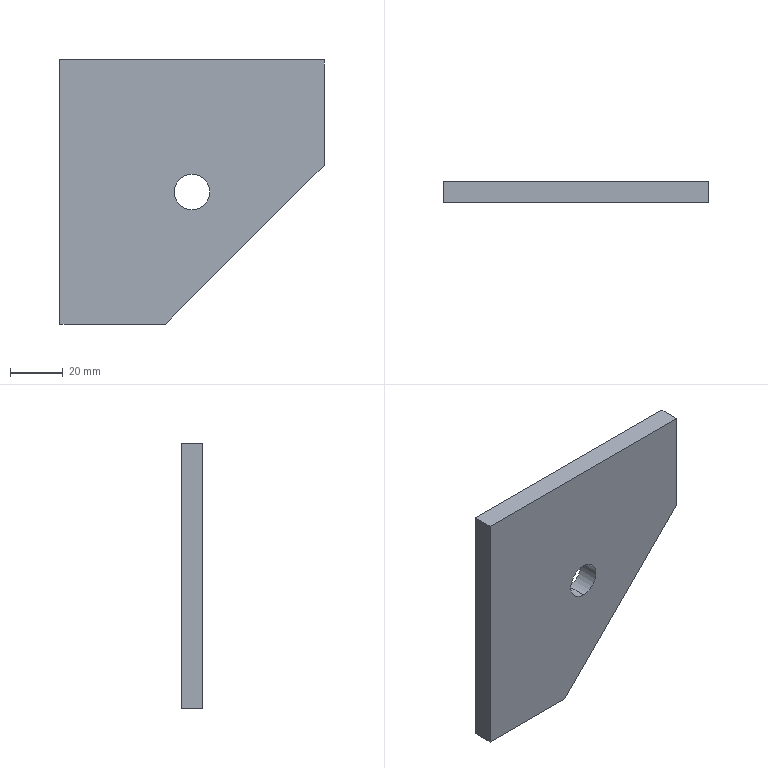Part | SolidWorks | features Extrusion 1, HoleWzd 1 | 1 solid | 9 faces | box 100 x 8 x 100 mm | volume 64455 mm3 | plane 7 | cylinder 2 | commonest cylinder face diameters 13.5 x2
STEP:
#1=CARTESIAN_POINT('',(50.,0.,-43.25));
#2=VERTEX_POINT('',#1);
#3=CARTESIAN_POINT('',(50.,0.,-56.75));
#4=VERTEX_POINT('',#3);
#5=CARTESIAN_POINT('',(50.,0.,-50.));
#6=DIRECTION('',(0.,-1.,0.));
#7=DIRECTION('',(0.,0.,-1.));
#8=AXIS2_PLACEMENT_3D('',#5,#6,#7);
#9=CIRCLE('',#8,6.75);
#10=EDGE_CURVE('',#2,#4,#9,.T.);
#11=ORIENTED_EDGE('',*,*,#10,.T.);
#12=CARTESIAN_POINT('',(50.,8.,-56.75));
#13=VERTEX_POINT('',#12);
#14=CARTESIAN_POINT('',(50.,8.,-56.75));
#15=DIRECTION('',(0.,1.,0.));
#16=VECTOR('',#15,1000.);
#17=LINE('',#14,#16);
#18=EDGE_CURVE('',#4,#13,#17,.T.);
#19=ORIENTED_EDGE('',*,*,#18,.T.);
#20=CARTESIAN_POINT('',(50.,8.,-43.25));
#21=VERTEX_POINT('',#20);
#22=CARTESIAN_POINT('',(50.,8.,-50.));
#23=DIRECTION('',(0.,1.,0.));
#24=DIRECTION('',(0.,0.,1.));
#25=AXIS2_PLACEMENT_3D('',#22,#23,#24);
#26=CIRCLE('',#25,6.75);
#27=EDGE_CURVE('',#13,#21,#26,.T.);
#28=ORIENTED_EDGE('',*,*,#27,.T.);
#29=CARTESIAN_POINT('',(50.,8.,-43.25));
#30=DIRECTION('',(0.,1.,0.));
#31=VECTOR('',#30,1000.);
#32=LINE('',#29,#31);
#33=EDGE_CURVE('',#2,#21,#32,.T.);
#34=ORIENTED_EDGE('',*,*,#33,.F.);
#35=EDGE_LOOP('',(#11,#19,#28,#34));
#36=FACE_OUTER_BOUND('',#35,.T.);
#37=CARTESIAN_POINT('',(50.,8.,-50.));
#38=DIRECTION('',(0.,1.,0.));
#39=DIRECTION('',(0.,0.,1.));
#40=AXIS2_PLACEMENT_3D('',#37,#38,#39);
#41=CYLINDRICAL_SURFACE('',#40,6.75);
#42=ADVANCED_FACE('',(#36),#41,.F.);
#43=CARTESIAN_POINT('',(0.,0.,-100.));
#44=VERTEX_POINT('',#43);
#45=CARTESIAN_POINT('',(0.,0.,0.));
#46=VERTEX_POINT('',#45);
#47=CARTESIAN_POINT('',(0.,0.,0.));
#48=DIRECTION('',(0.,0.,1.));
#49=VECTOR('',#48,1000.);
#50=LINE('',#47,#49);
#51=EDGE_CURVE('',#44,#46,#50,.T.);
#52=ORIENTED_EDGE('',*,*,#51,.T.);
#53=CARTESIAN_POINT('',(0.,8.,0.));
#54=VERTEX_POINT('',#53);
#55=CARTESIAN_POINT('',(0.,8.,0.));
#56=DIRECTION('',(0.,-1.,0.));
#57=VECTOR('',#56,1000.);
#58=LINE('',#55,#57);
#59=EDGE_CURVE('',#54,#46,#58,.T.);
#60=ORIENTED_EDGE('',*,*,#59,.F.);
#61=CARTESIAN_POINT('',(0.,8.,-100.));
#62=VERTEX_POINT('',#61);
#63=CARTESIAN_POINT('',(0.,8.,0.));
#64=DIRECTION('',(0.,0.,1.));
#65=VECTOR('',#64,1000.);
#66=LINE('',#63,#65);
#67=EDGE_CURVE('',#62,#54,#66,.T.);
#68=ORIENTED_EDGE('',*,*,#67,.F.);
#69=CARTESIAN_POINT('',(0.,8.,-100.));
#70=DIRECTION('',(0.,-1.,0.));
#71=VECTOR('',#70,1000.);
#72=LINE('',#69,#71);
#73=EDGE_CURVE('',#62,#44,#72,.T.);
#74=ORIENTED_EDGE('',*,*,#73,.T.);
#75=EDGE_LOOP('',(#52,#60,#68,#74));
#76=FACE_OUTER_BOUND('',#75,.T.);
#77=CARTESIAN_POINT('',(0.,8.,0.));
#78=DIRECTION('',(1.,0.,0.));
#79=DIRECTION('',(0.,0.,-1.));
#80=AXIS2_PLACEMENT_3D('',#77,#78,#79);
#81=PLANE('',#80);
#82=ADVANCED_FACE('',(#76),#81,.F.);
#83=CARTESIAN_POINT('',(100.,0.,0.));
#84=VERTEX_POINT('',#83);
#85=CARTESIAN_POINT('',(0.,0.,0.));
#86=DIRECTION('',(1.,0.,0.));
#87=VECTOR('',#86,1000.);
#88=LINE('',#85,#87);
#89=EDGE_CURVE('',#46,#84,#88,.T.);
#90=ORIENTED_EDGE('',*,*,#89,.T.);
#91=CARTESIAN_POINT('',(100.,8.,0.));
#92=VERTEX_POINT('',#91);
#93=CARTESIAN_POINT('',(100.,8.,0.));
#94=DIRECTION('',(0.,-1.,0.));
#95=VECTOR('',#94,1000.);
#96=LINE('',#93,#95);
#97=EDGE_CURVE('',#92,#84,#96,.T.);
#98=ORIENTED_EDGE('',*,*,#97,.F.);
#99=CARTESIAN_POINT('',(0.,8.,0.));
#100=DIRECTION('',(1.,0.,0.));
#101=VECTOR('',#100,1000.);
#102=LINE('',#99,#101);
#103=EDGE_CURVE('',#54,#92,#102,.T.);
#104=ORIENTED_EDGE('',*,*,#103,.F.);
#105=ORIENTED_EDGE('',*,*,#59,.T.);
#106=EDGE_LOOP('',(#90,#98,#104,#105));
#107=FACE_OUTER_BOUND('',#106,.T.);
#108=CARTESIAN_POINT('',(0.,8.,0.));
#109=DIRECTION('',(0.,0.,-1.));
#110=DIRECTION('',(-1.,0.,0.));
#111=AXIS2_PLACEMENT_3D('',#108,#109,#110);
#112=PLANE('',#111);
#113=ADVANCED_FACE('',(#107),#112,.F.);
#114=CARTESIAN_POINT('',(100.,0.,-40.));
#115=VERTEX_POINT('',#114);
#116=CARTESIAN_POINT('',(100.,0.,0.));
#117=DIRECTION('',(0.,0.,-1.));
#118=VECTOR('',#117,1000.);
#119=LINE('',#116,#118);
#120=EDGE_CURVE('',#84,#115,#119,.T.);
#121=ORIENTED_EDGE('',*,*,#120,.T.);
#122=CARTESIAN_POINT('',(100.,8.,-40.));
#123=VERTEX_POINT('',#122);
#124=CARTESIAN_POINT('',(100.,8.,-40.));
#125=DIRECTION('',(0.,-1.,0.));
#126=VECTOR('',#125,1000.);
#127=LINE('',#124,#126);
#128=EDGE_CURVE('',#123,#115,#127,.T.);
#129=ORIENTED_EDGE('',*,*,#128,.F.);
#130=CARTESIAN_POINT('',(100.,8.,0.));
#131=DIRECTION('',(0.,0.,-1.));
#132=VECTOR('',#131,1000.);
#133=LINE('',#130,#132);
#134=EDGE_CURVE('',#92,#123,#133,.T.);
#135=ORIENTED_EDGE('',*,*,#134,.F.);
#136=ORIENTED_EDGE('',*,*,#97,.T.);
#137=EDGE_LOOP('',(#121,#129,#135,#136));
#138=FACE_OUTER_BOUND('',#137,.T.);
#139=CARTESIAN_POINT('',(100.,8.,0.));
#140=DIRECTION('',(-1.,0.,0.));
#141=DIRECTION('',(0.,0.,1.));
#142=AXIS2_PLACEMENT_3D('',#139,#140,#141);
#143=PLANE('',#142);
#144=ADVANCED_FACE('',(#138),#143,.F.);
#145=CARTESIAN_POINT('',(40.,0.,-100.));
#146=VERTEX_POINT('',#145);
#147=CARTESIAN_POINT('',(40.,0.,-100.));
#148=DIRECTION('',(-0.7071,0.,-0.7071));
#149=VECTOR('',#148,1000.);
#150=LINE('',#147,#149);
#151=EDGE_CURVE('',#115,#146,#150,.T.);
#152=ORIENTED_EDGE('',*,*,#151,.T.);
#153=CARTESIAN_POINT('',(40.,8.,-100.));
#154=VERTEX_POINT('',#153);
#155=CARTESIAN_POINT('',(40.,8.,-100.));
#156=DIRECTION('',(0.,-1.,0.));
#157=VECTOR('',#156,1000.);
#158=LINE('',#155,#157);
#159=EDGE_CURVE('',#154,#146,#158,.T.);
#160=ORIENTED_EDGE('',*,*,#159,.F.);
#161=CARTESIAN_POINT('',(40.,8.,-100.));
#162=DIRECTION('',(-0.7071,0.,-0.7071));
#163=VECTOR('',#162,1000.);
#164=LINE('',#161,#163);
#165=EDGE_CURVE('',#123,#154,#164,.T.);
#166=ORIENTED_EDGE('',*,*,#165,.F.);
#167=ORIENTED_EDGE('',*,*,#128,.T.);
#168=EDGE_LOOP('',(#152,#160,#166,#167));
#169=FACE_OUTER_BOUND('',#168,.T.);
#170=CARTESIAN_POINT('',(40.,8.,-100.));
#171=DIRECTION('',(-0.7071,0.,0.7071));
#172=DIRECTION('',(0.7071,0.,0.7071));
#173=AXIS2_PLACEMENT_3D('',#170,#171,#172);
#174=PLANE('',#173);
#175=ADVANCED_FACE('',(#169),#174,.F.);
#176=CARTESIAN_POINT('',(0.,0.,-100.));
#177=DIRECTION('',(-1.,0.,0.));
#178=VECTOR('',#177,1000.);
#179=LINE('',#176,#178);
#180=EDGE_CURVE('',#146,#44,#179,.T.);
#181=ORIENTED_EDGE('',*,*,#180,.T.);
#182=ORIENTED_EDGE('',*,*,#73,.F.);
#183=CARTESIAN_POINT('',(0.,8.,-100.));
#184=DIRECTION('',(-1.,0.,0.));
#185=VECTOR('',#184,1000.);
#186=LINE('',#183,#185);
#187=EDGE_CURVE('',#154,#62,#186,.T.);
#188=ORIENTED_EDGE('',*,*,#187,.F.);
#189=ORIENTED_EDGE('',*,*,#159,.T.);
#190=EDGE_LOOP('',(#181,#182,#188,#189));
#191=FACE_OUTER_BOUND('',#190,.T.);
#192=CARTESIAN_POINT('',(0.,8.,-100.));
#193=DIRECTION('',(0.,0.,1.));
#194=DIRECTION('',(1.,0.,0.));
#195=AXIS2_PLACEMENT_3D('',#192,#193,#194);
#196=PLANE('',#195);
#197=ADVANCED_FACE('',(#191),#196,.F.);
#198=CARTESIAN_POINT('',(50.,8.,-50.));
#199=DIRECTION('',(0.,1.,0.));
#200=DIRECTION('',(0.,0.,1.));
#201=AXIS2_PLACEMENT_3D('',#198,#199,#200);
#202=CIRCLE('',#201,6.75);
#203=EDGE_CURVE('',#21,#13,#202,.T.);
#204=ORIENTED_EDGE('',*,*,#203,.F.);
#205=ORIENTED_EDGE('',*,*,#27,.F.);
#206=EDGE_LOOP('',(#204,#205));
#207=FACE_BOUND('',#206,.T.);
#208=ORIENTED_EDGE('',*,*,#67,.T.);
#209=ORIENTED_EDGE('',*,*,#103,.T.);
#210=ORIENTED_EDGE('',*,*,#134,.T.);
#211=ORIENTED_EDGE('',*,*,#165,.T.);
#212=ORIENTED_EDGE('',*,*,#187,.T.);
#213=EDGE_LOOP('',(#208,#209,#210,#211,#212));
#214=FACE_OUTER_BOUND('',#213,.T.);
#215=CARTESIAN_POINT('',(0.,8.,0.));
#216=DIRECTION('',(0.,-1.,0.));
#217=DIRECTION('',(0.,0.,-1.));
#218=AXIS2_PLACEMENT_3D('',#215,#216,#217);
#219=PLANE('',#218);
#220=ADVANCED_FACE('',(#207,#214),#219,.F.);
#221=ORIENTED_EDGE('',*,*,#10,.F.);
#222=CARTESIAN_POINT('',(50.,0.,-50.));
#223=DIRECTION('',(0.,-1.,0.));
#224=DIRECTION('',(0.,0.,-1.));
#225=AXIS2_PLACEMENT_3D('',#222,#223,#224);
#226=CIRCLE('',#225,6.75);
#227=EDGE_CURVE('',#4,#2,#226,.T.);
#228=ORIENTED_EDGE('',*,*,#227,.F.);
#229=EDGE_LOOP('',(#221,#228));
#230=FACE_BOUND('',#229,.T.);
#231=ORIENTED_EDGE('',*,*,#51,.F.);
#232=ORIENTED_EDGE('',*,*,#180,.F.);
#233=ORIENTED_EDGE('',*,*,#151,.F.);
#234=ORIENTED_EDGE('',*,*,#120,.F.);
#235=ORIENTED_EDGE('',*,*,#89,.F.);
#236=EDGE_LOOP('',(#231,#232,#233,#234,#235));
#237=FACE_OUTER_BOUND('',#236,.T.);
#238=CARTESIAN_POINT('',(0.,0.,0.));
#239=DIRECTION('',(0.,-1.,0.));
#240=DIRECTION('',(0.,0.,-1.));
#241=AXIS2_PLACEMENT_3D('',#238,#239,#240);
#242=PLANE('',#241);
#243=ADVANCED_FACE('',(#230,#237),#242,.T.);
#244=ORIENTED_EDGE('',*,*,#18,.F.);
#245=ORIENTED_EDGE('',*,*,#227,.T.);
#246=ORIENTED_EDGE('',*,*,#33,.T.);
#247=ORIENTED_EDGE('',*,*,#203,.T.);
#248=EDGE_LOOP('',(#244,#245,#246,#247));
#249=FACE_OUTER_BOUND('',#248,.T.);
#250=CARTESIAN_POINT('',(50.,8.,-50.));
#251=DIRECTION('',(0.,1.,0.));
#252=DIRECTION('',(0.,0.,1.));
#253=AXIS2_PLACEMENT_3D('',#250,#251,#252);
#254=CYLINDRICAL_SURFACE('',#253,6.75);
#255=ADVANCED_FACE('',(#249),#254,.F.);
#256=CLOSED_SHELL('',(#42,#82,#113,#144,#175,#197,#220,#243,#255));
#257=MANIFOLD_SOLID_BREP('',#256);
#258=CARTESIAN_POINT('',(0.,0.,0.));
#259=DIRECTION('',(0.,0.,1.));
#260=DIRECTION('',(1.,0.,0.));
#261=AXIS2_PLACEMENT_3D('',#258,#259,#260);
#262=(LENGTH_UNIT()NAMED_UNIT(*)SI_UNIT(.MILLI.,.METRE.));
#263=UNCERTAINTY_MEASURE_WITH_UNIT(LENGTH_MEASURE(0.00001),#262,'','');
#264=(NAMED_UNIT(*)PLANE_ANGLE_UNIT()SI_UNIT($,.RADIAN.));
#265=(NAMED_UNIT(*)SI_UNIT($,.STERADIAN.)SOLID_ANGLE_UNIT());
#266=(GEOMETRIC_REPRESENTATION_CONTEXT(3)GLOBAL_UNCERTAINTY_ASSIGNED_CONTEXT((#263))GLOBAL_UNIT_ASSIGNED_CONTEXT((#262,#264,#265))REPRESENTATION_CONTEXT('',''));
#267=ADVANCED_BREP_SHAPE_REPRESENTATION('',(#257,#261),#266);